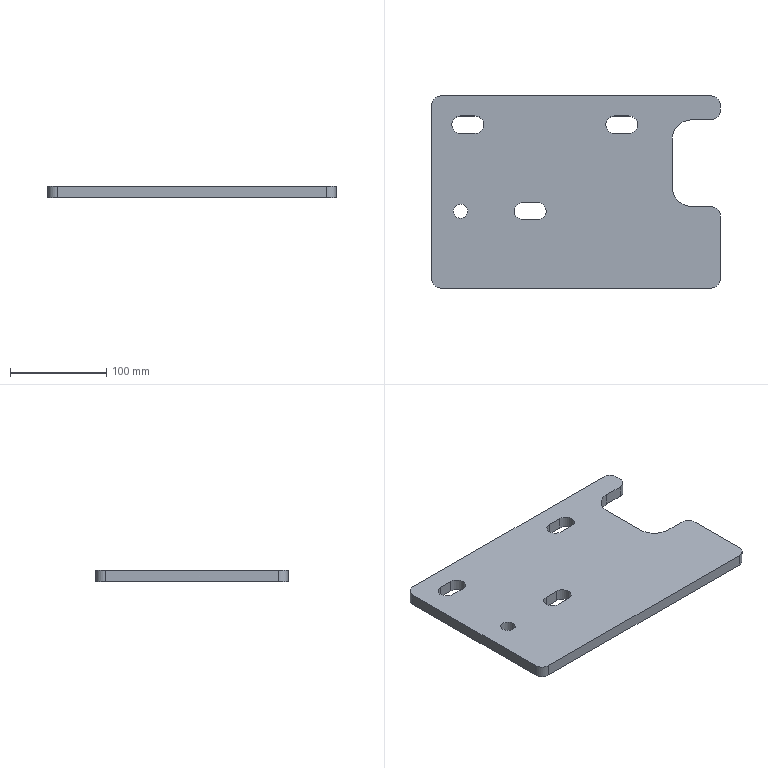Part | STEP file | Sheet5 | 1 solid | 31 faces | box 300 x 200 x 12 mm | volume 645514 mm3 | plane 16 | cylinder 15 | commonest cylinder face diameters 18 x6 20 x6 40 x2 15 x1